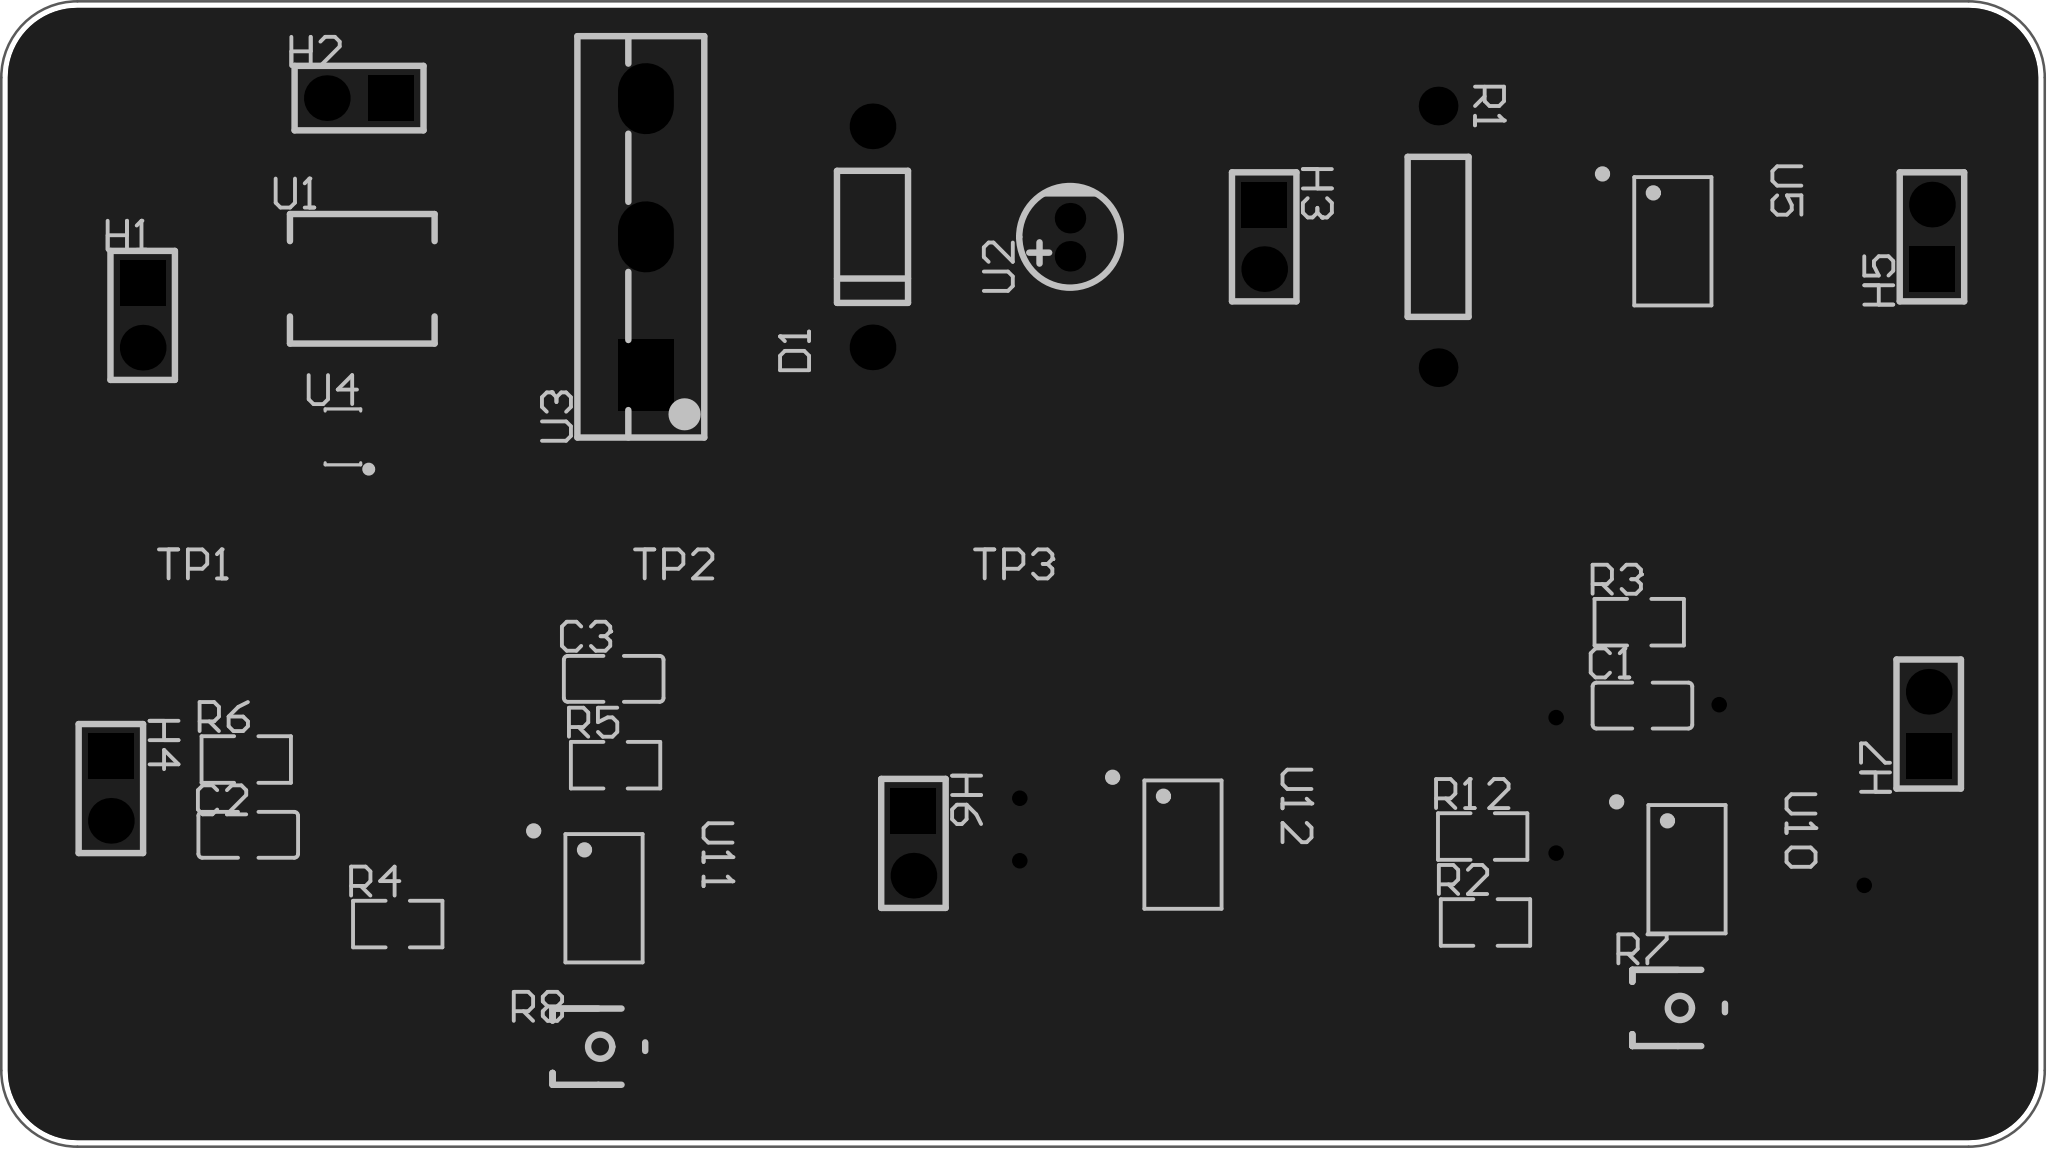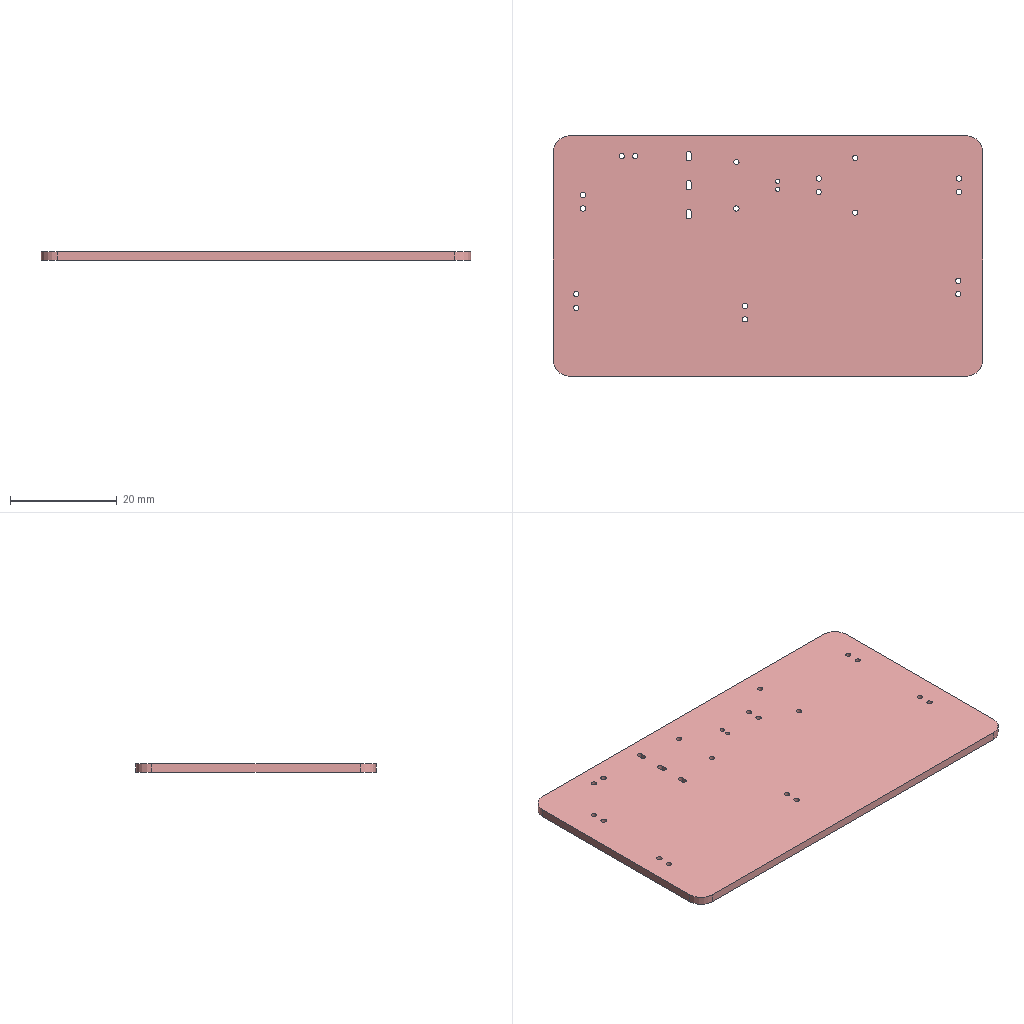Circuit board layout | Altium Designer | box 80.5 x 45.1 x 1.6 mm
Layer stack:
# Altium Designer layer stack of  (unit mm; dielectric type: 0 none, 1 core, 2 prepreg, 3 surface material)
index,name,kind,layer,copper_thickness_mm,dielectric_type,dielectric_thickness_mm,dielectric_material,dielectric_constant
0,Top Paste Mask Layer,other,,,,,,
1,Top Silkscreen Layer,other,,,,,,
2,Top Solder Mask Layer,dielectric,,,3,0.01,,3.3
3,Top Layer,copper,Top Layer,0.035,,,,
4,Dielectric1,dielectric,,,3,1.51,FR4,4.5
5,Bottom Layer,copper,Bottom Layer,0.035,,,,
6,Bottom Solder Mask Layer,dielectric,,,3,0.01,,3.3
7,Bottom Silkscreen Layer,other,,,,,,
8,Bottom Paste Mask Layer,other,,,,,,
# drill layer pairs: low layer,high layer
drill_pair,Top Layer,Bottom Layer
Part placement:
Designator,Comment,Layer,Footprint,Center-X(mm),Center-Y(mm),Rotation
C1,100nF,TopLayer,C0805,143.405,96.103,0
C2,100nF,TopLayer,C0805,88.471,91.017,180
C3,1nF,TopLayer,C0805,102.87,97.155,0
D1,,TopLayer,DO_1N4007,113.068,114.554,90
H1,,TopLayer,HDR-TH_2P-P2.54-V-M-1,84.312,111.462,270
H2,,TopLayer,HDR-TH_2P-P2.54-V-M-1,92.837,120.015,180
H3,,TopLayer,HDR-TH_2P-P2.54-V-M-1,128.502,114.554,270
H4,,TopLayer,HDR-TH_2P-P2.54-V-M-1,83.058,92.837,270
H5,,TopLayer,HDR-TH_2P-P2.54-V-M-1,154.813,114.554,90
H6,,TopLayer,HDR-TH_2P-P2.54-V-M-1,114.681,90.678,270
H7,,TopLayer,HDR-TH_2P-P2.54-V-M-1,154.686,95.377,90
R1,10kΩ,TopLayer,Res_1/4W,135.354,114.554,270
R2,10kΩ,TopLayer,R0805,137.221,87.566,0
R3,1MΩ,TopLayer,R0805,143.278,99.385,0
R4,10kΩ,TopLayer,R0805,94.361,87.503,0
R5,10kΩ,TopLayer,R0805,102.945,93.757,0
R6,100Ω,TopLayer,R0805,88.392,93.98,0
R7,100kΩ,TopLayer,RES-ADJ-SMD_VG039NCH,144.907,84.201,0
R8,100kΩ,TopLayer,RES-ADJ-SMD_VG039NCH,102.362,82.677,0
R12,10kΩ,TopLayer,R0805,137.111,90.949,0
TP1,,TopLayer,Test-Point-0.5mm,85.201,100.731,0
TP2,,TopLayer,Test-Point-0.5mm,103.961,100.731,0
TP3,,TopLayer,Test-Point-0.5mm,117.358,100.731,0
U1,功率电感(贴片),CKST0502-10uH/M,10uH,±20%,3A,封装5.7mm*5.1mm*2.0mm,岑科,RoHS,TopLayer,IND-SMD_L5.7-W5.1,92.964,112.903,0
U2,10uF,TopLayer,CAP-TH_BD4.0-P1.50-D0.8-FD,120.849,114.539,90
U3,HY5204,TopLayer,TO-247-3_L15.8-W5.0-P5.44-L-1,104.14,114.554,90
U4,SN74LVC2G04DCKR,TopLayer,SOT-363_L2.0-W1.3-P0.65-LS2.1-BR,92.202,106.68,0
U5,NE5532DR,TopLayer,SOIC-8_L4.9-W3.9-P1.27-LS6.0-BL,144.604,114.379,270
U10,UA741CDT,TopLayer,SOIC-8_L4.9-W3.9-P1.27-LS6.0-BL,145.161,89.662,270
U11,UA741CDT,TopLayer,SOIC-8_L4.9-W3.9-P1.27-LS6.0-BL,102.489,88.519,270
U12,NE5532DR,TopLayer,SOIC-8_L4.9-W3.9-P1.27-LS6.0-BL,125.301,90.63,270
Pad and via stacks:
# Altium Designer via and pad stacks of  (unit mm). Each distinct definition once, with the count of objects using it.
# via: kind,start_layer,end_layer,hole_mm,diameter_mm,mode(0 simple;1 top-mid-bottom;2 full stack),diameter_per_layer,count,example_net
# pad: kind,layer,hole_mm,hole_type(0 round;1 square;2 slot),plating,top_size,top_shape(1 round;2 rect;3 octagon;9 rounded rect),mid_size,bottom_size,mode,footprint,size_per_layer,count,example
pad,Top Layer,0,0,plated,1.41x1.35,2,1.41x1.35,1.41x1.35,0,C0805,,6,C1.2
pad,Top Layer,0,0,plated,1.133x1.377,2,1.133x1.377,1.133x1.377,0,R0805,,12,R2.2
pad,Top Layer,0,0,plated,1.6x1.6,2,1.6x1.6,1.6x1.6,0,RES-ADJ-SMD_VG039NCH,,2,R7.2
pad,Top Layer,0,0,plated,1.2x1.5,2,1.2x1.5,1.2x1.5,0,RES-ADJ-SMD_VG039NCH,,4,R7.3
pad,Top Layer,0,0,plated,0.5x0.5,1,0.5x0.5,0.5x0.5,0,Test-Point-0.5mm,,3,TP1.1
pad,Top Layer,0,0,plated,2x2.5,2,2x2.5,2x2.5,0,IND-SMD_L5.7-W5.1,,2,U1.1
pad,Top Layer,0,0,plated,0.4x0.9,2,0.4x0.9,0.4x0.9,0,SOT-363_L2.0-W1.3-P0.65-LS2.1-BR,,6,U4.2
pad,Top Layer,0,0,plated,0.588x2.045,1,0.588x2.045,0.588x2.045,0,SOIC-8_L4.9-W3.9-P1.27-LS6.0-BL,,32,U5.1
pad,Multi-Layer,1,0,plated,1.8x1.8,1,1.8x1.8,1.8x1.8,0,DO_1N4007,,2,D1.1
pad,Multi-Layer,1,0,plated,1.8x1.8,1,1.8x1.8,1.8x1.8,0,HDR-TH_2P-P2.54-V-M-1,,7,H1.2
pad,Multi-Layer,1,0,plated,1.8x1.8,2,1.8x1.8,1.8x1.8,0,HDR-TH_2P-P2.54-V-M-1,,7,H1.1
pad,Multi-Layer,1,0,plated,1.524x1.524,1,1.524x1.524,1.524x1.524,0,Res_1/4W,,2,R1.1
pad,Multi-Layer,0.8,0,plated,1.2x1.2,1,1.2x1.2,1.2x1.2,0,CAP-TH_BD4.0-P1.50-D0.8-FD,,2,U2.2
pad,Multi-Layer,1,2,plated,2.8x2.2,1,2.8x2.2,2.8x2.2,0,TO-247-3_L15.8-W5.0-P5.44-L-1,,2,U3.3
pad,Multi-Layer,1,2,plated,2.8x2.2,2,2.8x2.2,2.8x2.2,0,TO-247-3_L15.8-W5.0-P5.44-L-1,,1,U3.1
via,Top Layer,Bottom Layer,0.3048,0.6096,0,,5,$1N3432
via,Top Layer,Bottom Layer,0.3048,0.61,0,,1,$1N3429
Copper pours:
name,layer,net,type(0 solid;1 hatched;2 none)
Top Layer-GND,Top Layer,GND,0
Bottom Layer-GND,Bottom Layer,GND,0